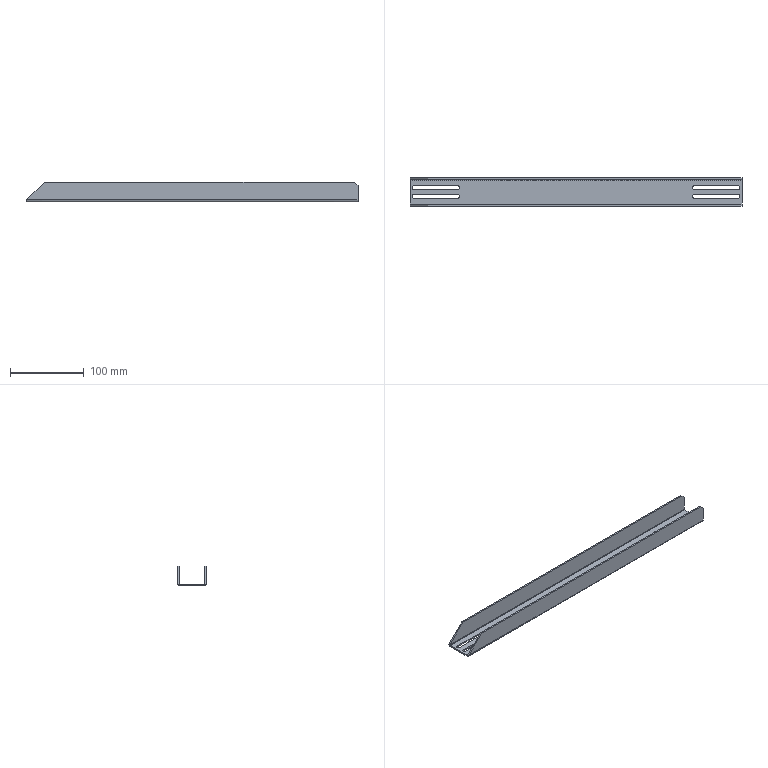Part | NX | 1 solid | 40 faces | box 450 x 38 x 27 mm | volume 74271 mm3 | plane 28 | cylinder 12 | commonest cylinder face diameters 4.5 x8 1.473 x2 5.473 x2
STEP:
#1=CARTESIAN_POINT('',(-160.,-3.75,-2.));
#2=VERTEX_POINT('',#1);
#3=CARTESIAN_POINT('',(-220.,-3.75,-2.));
#4=VERTEX_POINT('',#3);
#5=CARTESIAN_POINT('',(0.,-3.75,-2.));
#6=DIRECTION('',(-1.,0.,0.));
#7=VECTOR('',#6,1000.);
#8=LINE('',#5,#7);
#9=EDGE_CURVE('',#2,#4,#8,.T.);
#10=ORIENTED_EDGE('',*,*,#9,.T.);
#11=CARTESIAN_POINT('',(-220.,-8.25,-2.));
#12=VERTEX_POINT('',#11);
#13=CARTESIAN_POINT('',(-220.,-6.,-2.));
#14=DIRECTION('',(0.,0.,-1.));
#15=DIRECTION('',(-1.,0.,0.));
#16=AXIS2_PLACEMENT_3D('',#13,#14,#15);
#17=CIRCLE('',#16,2.25);
#18=EDGE_CURVE('',#4,#12,#17,.F.);
#19=ORIENTED_EDGE('',*,*,#18,.T.);
#20=CARTESIAN_POINT('',(-160.,-8.25,-2.));
#21=VERTEX_POINT('',#20);
#22=CARTESIAN_POINT('',(0.,-8.25,-2.));
#23=DIRECTION('',(1.,0.,0.));
#24=VECTOR('',#23,1000.);
#25=LINE('',#22,#24);
#26=EDGE_CURVE('',#12,#21,#25,.T.);
#27=ORIENTED_EDGE('',*,*,#26,.T.);
#28=CARTESIAN_POINT('',(-160.,-6.,-2.));
#29=DIRECTION('',(0.,0.,-1.));
#30=DIRECTION('',(-1.,0.,0.));
#31=AXIS2_PLACEMENT_3D('',#28,#29,#30);
#32=CIRCLE('',#31,2.25);
#33=EDGE_CURVE('',#21,#2,#32,.F.);
#34=ORIENTED_EDGE('',*,*,#33,.T.);
#35=EDGE_LOOP('',(#10,#19,#27,#34));
#36=FACE_BOUND('',#35,.T.);
#37=CARTESIAN_POINT('',(-220.,3.75,-2.));
#38=VERTEX_POINT('',#37);
#39=CARTESIAN_POINT('',(-220.,8.25,-2.));
#40=VERTEX_POINT('',#39);
#41=CARTESIAN_POINT('',(-220.,6.,-2.));
#42=DIRECTION('',(0.,0.,-1.));
#43=DIRECTION('',(-1.,0.,0.));
#44=AXIS2_PLACEMENT_3D('',#41,#42,#43);
#45=CIRCLE('',#44,2.25);
#46=EDGE_CURVE('',#38,#40,#45,.T.);
#47=ORIENTED_EDGE('',*,*,#46,.F.);
#48=CARTESIAN_POINT('',(-160.,3.75,-2.));
#49=VERTEX_POINT('',#48);
#50=CARTESIAN_POINT('',(0.,3.75,-2.));
#51=DIRECTION('',(-1.,0.,0.));
#52=VECTOR('',#51,1000.);
#53=LINE('',#50,#52);
#54=EDGE_CURVE('',#49,#38,#53,.T.);
#55=ORIENTED_EDGE('',*,*,#54,.F.);
#56=CARTESIAN_POINT('',(-160.,8.25,-2.));
#57=VERTEX_POINT('',#56);
#58=CARTESIAN_POINT('',(-160.,6.,-2.));
#59=DIRECTION('',(0.,0.,-1.));
#60=DIRECTION('',(-1.,0.,0.));
#61=AXIS2_PLACEMENT_3D('',#58,#59,#60);
#62=CIRCLE('',#61,2.25);
#63=EDGE_CURVE('',#57,#49,#62,.T.);
#64=ORIENTED_EDGE('',*,*,#63,.F.);
#65=CARTESIAN_POINT('',(0.,8.25,-2.));
#66=DIRECTION('',(1.,0.,0.));
#67=VECTOR('',#66,1000.);
#68=LINE('',#65,#67);
#69=EDGE_CURVE('',#40,#57,#68,.T.);
#70=ORIENTED_EDGE('',*,*,#69,.F.);
#71=EDGE_LOOP('',(#47,#55,#64,#70));
#72=FACE_BOUND('',#71,.T.);
#73=CARTESIAN_POINT('',(-225.,16.263,-2.));
#74=VERTEX_POINT('',#73);
#75=CARTESIAN_POINT('',(-225.,-16.263,-2.));
#76=VERTEX_POINT('',#75);
#77=CARTESIAN_POINT('',(-225.,-17.,-2.));
#78=DIRECTION('',(0.,-1.,0.));
#79=VECTOR('',#78,1000.);
#80=LINE('',#77,#79);
#81=EDGE_CURVE('',#74,#76,#80,.T.);
#82=ORIENTED_EDGE('',*,*,#81,.F.);
#83=CARTESIAN_POINT('',(225.,16.263,-2.));
#84=VERTEX_POINT('',#83);
#85=CARTESIAN_POINT('',(-225.,16.263,-2.));
#86=DIRECTION('',(-1.,0.,0.));
#87=VECTOR('',#86,1000.);
#88=LINE('',#85,#87);
#89=EDGE_CURVE('',#74,#84,#88,.F.);
#90=ORIENTED_EDGE('',*,*,#89,.T.);
#91=CARTESIAN_POINT('',(225.,-16.263,-2.));
#92=VERTEX_POINT('',#91);
#93=CARTESIAN_POINT('',(225.,-17.,-2.));
#94=DIRECTION('',(0.,1.,0.));
#95=VECTOR('',#94,1000.);
#96=LINE('',#93,#95);
#97=EDGE_CURVE('',#92,#84,#96,.T.);
#98=ORIENTED_EDGE('',*,*,#97,.F.);
#99=CARTESIAN_POINT('',(225.,-16.263,-2.));
#100=DIRECTION('',(1.,0.,0.));
#101=VECTOR('',#100,1000.);
#102=LINE('',#99,#101);
#103=EDGE_CURVE('',#92,#76,#102,.F.);
#104=ORIENTED_EDGE('',*,*,#103,.T.);
#105=EDGE_LOOP('',(#82,#90,#98,#104));
#106=FACE_BOUND('',#105,.T.);
#107=CARTESIAN_POINT('',(220.,-3.75,-2.));
#108=VERTEX_POINT('',#107);
#109=CARTESIAN_POINT('',(220.,-8.25,-2.));
#110=VERTEX_POINT('',#109);
#111=CARTESIAN_POINT('',(220.,-6.,-2.));
#112=DIRECTION('',(0.,0.,-1.));
#113=DIRECTION('',(-1.,0.,0.));
#114=AXIS2_PLACEMENT_3D('',#111,#112,#113);
#115=CIRCLE('',#114,2.25);
#116=EDGE_CURVE('',#108,#110,#115,.T.);
#117=ORIENTED_EDGE('',*,*,#116,.F.);
#118=CARTESIAN_POINT('',(160.,-3.75,-2.));
#119=VERTEX_POINT('',#118);
#120=CARTESIAN_POINT('',(0.,-3.75,-2.));
#121=DIRECTION('',(1.,0.,0.));
#122=VECTOR('',#121,1000.);
#123=LINE('',#120,#122);
#124=EDGE_CURVE('',#119,#108,#123,.T.);
#125=ORIENTED_EDGE('',*,*,#124,.F.);
#126=CARTESIAN_POINT('',(160.,-8.25,-2.));
#127=VERTEX_POINT('',#126);
#128=CARTESIAN_POINT('',(160.,-6.,-2.));
#129=DIRECTION('',(0.,0.,-1.));
#130=DIRECTION('',(-1.,0.,0.));
#131=AXIS2_PLACEMENT_3D('',#128,#129,#130);
#132=CIRCLE('',#131,2.25);
#133=EDGE_CURVE('',#127,#119,#132,.T.);
#134=ORIENTED_EDGE('',*,*,#133,.F.);
#135=CARTESIAN_POINT('',(0.,-8.25,-2.));
#136=DIRECTION('',(-1.,0.,0.));
#137=VECTOR('',#136,1000.);
#138=LINE('',#135,#137);
#139=EDGE_CURVE('',#110,#127,#138,.T.);
#140=ORIENTED_EDGE('',*,*,#139,.F.);
#141=EDGE_LOOP('',(#117,#125,#134,#140));
#142=FACE_BOUND('',#141,.T.);
#143=CARTESIAN_POINT('',(160.,3.75,-2.));
#144=VERTEX_POINT('',#143);
#145=CARTESIAN_POINT('',(220.,3.75,-2.));
#146=VERTEX_POINT('',#145);
#147=CARTESIAN_POINT('',(0.,3.75,-2.));
#148=DIRECTION('',(1.,0.,0.));
#149=VECTOR('',#148,1000.);
#150=LINE('',#147,#149);
#151=EDGE_CURVE('',#144,#146,#150,.T.);
#152=ORIENTED_EDGE('',*,*,#151,.T.);
#153=CARTESIAN_POINT('',(220.,8.25,-2.));
#154=VERTEX_POINT('',#153);
#155=CARTESIAN_POINT('',(220.,6.,-2.));
#156=DIRECTION('',(0.,0.,-1.));
#157=DIRECTION('',(-1.,0.,0.));
#158=AXIS2_PLACEMENT_3D('',#155,#156,#157);
#159=CIRCLE('',#158,2.25);
#160=EDGE_CURVE('',#146,#154,#159,.F.);
#161=ORIENTED_EDGE('',*,*,#160,.T.);
#162=CARTESIAN_POINT('',(160.,8.25,-2.));
#163=VERTEX_POINT('',#162);
#164=CARTESIAN_POINT('',(0.,8.25,-2.));
#165=DIRECTION('',(-1.,0.,0.));
#166=VECTOR('',#165,1000.);
#167=LINE('',#164,#166);
#168=EDGE_CURVE('',#154,#163,#167,.T.);
#169=ORIENTED_EDGE('',*,*,#168,.T.);
#170=CARTESIAN_POINT('',(160.,6.,-2.));
#171=DIRECTION('',(0.,0.,-1.));
#172=DIRECTION('',(-1.,0.,0.));
#173=AXIS2_PLACEMENT_3D('',#170,#171,#172);
#174=CIRCLE('',#173,2.25);
#175=EDGE_CURVE('',#163,#144,#174,.F.);
#176=ORIENTED_EDGE('',*,*,#175,.T.);
#177=EDGE_LOOP('',(#152,#161,#169,#176));
#178=FACE_BOUND('',#177,.T.);
#179=CARTESIAN_POINT('',(0.,0.,-2.));
#180=DIRECTION('',(0.,0.,-1.));
#181=DIRECTION('',(-1.,0.,0.));
#182=AXIS2_PLACEMENT_3D('',#179,#180,#181);
#183=PLANE('',#182);
#184=ADVANCED_FACE('',(#36,#72,#106,#142,#178),#183,.T.);
#185=CARTESIAN_POINT('',(-220.,-8.25,0.));
#186=VERTEX_POINT('',#185);
#187=CARTESIAN_POINT('',(-220.,-3.75,0.));
#188=VERTEX_POINT('',#187);
#189=CARTESIAN_POINT('',(-220.,-6.,0.));
#190=DIRECTION('',(0.,0.,-1.));
#191=DIRECTION('',(1.,0.,0.));
#192=AXIS2_PLACEMENT_3D('',#189,#190,#191);
#193=CIRCLE('',#192,2.25);
#194=EDGE_CURVE('',#186,#188,#193,.T.);
#195=ORIENTED_EDGE('',*,*,#194,.T.);
#196=CARTESIAN_POINT('',(-160.,-3.75,0.));
#197=VERTEX_POINT('',#196);
#198=CARTESIAN_POINT('',(-220.,-3.75,0.));
#199=DIRECTION('',(1.,0.,0.));
#200=VECTOR('',#199,1000.);
#201=LINE('',#198,#200);
#202=EDGE_CURVE('',#188,#197,#201,.T.);
#203=ORIENTED_EDGE('',*,*,#202,.T.);
#204=CARTESIAN_POINT('',(-160.,-8.25,0.));
#205=VERTEX_POINT('',#204);
#206=CARTESIAN_POINT('',(-160.,-6.,0.));
#207=DIRECTION('',(0.,0.,-1.));
#208=DIRECTION('',(1.,0.,0.));
#209=AXIS2_PLACEMENT_3D('',#206,#207,#208);
#210=CIRCLE('',#209,2.25);
#211=EDGE_CURVE('',#197,#205,#210,.T.);
#212=ORIENTED_EDGE('',*,*,#211,.T.);
#213=CARTESIAN_POINT('',(-220.,-8.25,0.));
#214=DIRECTION('',(-1.,0.,0.));
#215=VECTOR('',#214,1000.);
#216=LINE('',#213,#215);
#217=EDGE_CURVE('',#205,#186,#216,.T.);
#218=ORIENTED_EDGE('',*,*,#217,.T.);
#219=EDGE_LOOP('',(#195,#203,#212,#218));
#220=FACE_BOUND('',#219,.T.);
#221=CARTESIAN_POINT('',(-220.,3.75,0.));
#222=VERTEX_POINT('',#221);
#223=CARTESIAN_POINT('',(-160.,3.75,0.));
#224=VERTEX_POINT('',#223);
#225=CARTESIAN_POINT('',(-220.,3.75,0.));
#226=DIRECTION('',(1.,0.,0.));
#227=VECTOR('',#226,1000.);
#228=LINE('',#225,#227);
#229=EDGE_CURVE('',#222,#224,#228,.T.);
#230=ORIENTED_EDGE('',*,*,#229,.F.);
#231=CARTESIAN_POINT('',(-220.,8.25,0.));
#232=VERTEX_POINT('',#231);
#233=CARTESIAN_POINT('',(-220.,6.,0.));
#234=DIRECTION('',(0.,0.,1.));
#235=DIRECTION('',(1.,0.,0.));
#236=AXIS2_PLACEMENT_3D('',#233,#234,#235);
#237=CIRCLE('',#236,2.25);
#238=EDGE_CURVE('',#232,#222,#237,.T.);
#239=ORIENTED_EDGE('',*,*,#238,.F.);
#240=CARTESIAN_POINT('',(-160.,8.25,0.));
#241=VERTEX_POINT('',#240);
#242=CARTESIAN_POINT('',(-220.,8.25,0.));
#243=DIRECTION('',(-1.,0.,0.));
#244=VECTOR('',#243,1000.);
#245=LINE('',#242,#244);
#246=EDGE_CURVE('',#241,#232,#245,.T.);
#247=ORIENTED_EDGE('',*,*,#246,.F.);
#248=CARTESIAN_POINT('',(-160.,6.,0.));
#249=DIRECTION('',(0.,0.,1.));
#250=DIRECTION('',(1.,0.,0.));
#251=AXIS2_PLACEMENT_3D('',#248,#249,#250);
#252=CIRCLE('',#251,2.25);
#253=EDGE_CURVE('',#224,#241,#252,.T.);
#254=ORIENTED_EDGE('',*,*,#253,.F.);
#255=EDGE_LOOP('',(#230,#239,#247,#254));
#256=FACE_BOUND('',#255,.T.);
#257=CARTESIAN_POINT('',(-225.,16.263,0.));
#258=VERTEX_POINT('',#257);
#259=CARTESIAN_POINT('',(225.,16.263,0.));
#260=VERTEX_POINT('',#259);
#261=CARTESIAN_POINT('',(-225.,16.263,0.));
#262=DIRECTION('',(-1.,0.,0.));
#263=VECTOR('',#262,1000.);
#264=LINE('',#261,#263);
#265=EDGE_CURVE('',#258,#260,#264,.F.);
#266=ORIENTED_EDGE('',*,*,#265,.F.);
#267=CARTESIAN_POINT('',(-225.,-16.263,0.));
#268=VERTEX_POINT('',#267);
#269=CARTESIAN_POINT('',(-225.,-17.,0.));
#270=DIRECTION('',(0.,-1.,0.));
#271=VECTOR('',#270,1000.);
#272=LINE('',#269,#271);
#273=EDGE_CURVE('',#258,#268,#272,.T.);
#274=ORIENTED_EDGE('',*,*,#273,.T.);
#275=CARTESIAN_POINT('',(225.,-16.263,0.));
#276=VERTEX_POINT('',#275);
#277=CARTESIAN_POINT('',(225.,-16.263,0.));
#278=DIRECTION('',(1.,0.,0.));
#279=VECTOR('',#278,1000.);
#280=LINE('',#277,#279);
#281=EDGE_CURVE('',#276,#268,#280,.F.);
#282=ORIENTED_EDGE('',*,*,#281,.F.);
#283=CARTESIAN_POINT('',(225.,-17.,0.));
#284=DIRECTION('',(0.,1.,0.));
#285=VECTOR('',#284,1000.);
#286=LINE('',#283,#285);
#287=EDGE_CURVE('',#276,#260,#286,.T.);
#288=ORIENTED_EDGE('',*,*,#287,.T.);
#289=EDGE_LOOP('',(#266,#274,#282,#288));
#290=FACE_BOUND('',#289,.T.);
#291=CARTESIAN_POINT('',(220.,-3.75,0.));
#292=VERTEX_POINT('',#291);
#293=CARTESIAN_POINT('',(160.,-3.75,0.));
#294=VERTEX_POINT('',#293);
#295=CARTESIAN_POINT('',(220.,-3.75,0.));
#296=DIRECTION('',(-1.,0.,0.));
#297=VECTOR('',#296,1000.);
#298=LINE('',#295,#297);
#299=EDGE_CURVE('',#292,#294,#298,.T.);
#300=ORIENTED_EDGE('',*,*,#299,.F.);
#301=CARTESIAN_POINT('',(220.,-8.25,0.));
#302=VERTEX_POINT('',#301);
#303=CARTESIAN_POINT('',(220.,-6.,0.));
#304=DIRECTION('',(0.,0.,1.));
#305=DIRECTION('',(-1.,0.,0.));
#306=AXIS2_PLACEMENT_3D('',#303,#304,#305);
#307=CIRCLE('',#306,2.25);
#308=EDGE_CURVE('',#302,#292,#307,.T.);
#309=ORIENTED_EDGE('',*,*,#308,.F.);
#310=CARTESIAN_POINT('',(160.,-8.25,0.));
#311=VERTEX_POINT('',#310);
#312=CARTESIAN_POINT('',(220.,-8.25,0.));
#313=DIRECTION('',(1.,0.,0.));
#314=VECTOR('',#313,1000.);
#315=LINE('',#312,#314);
#316=EDGE_CURVE('',#311,#302,#315,.T.);
#317=ORIENTED_EDGE('',*,*,#316,.F.);
#318=CARTESIAN_POINT('',(160.,-6.,0.));
#319=DIRECTION('',(0.,0.,1.));
#320=DIRECTION('',(-1.,0.,0.));
#321=AXIS2_PLACEMENT_3D('',#318,#319,#320);
#322=CIRCLE('',#321,2.25);
#323=EDGE_CURVE('',#294,#311,#322,.T.);
#324=ORIENTED_EDGE('',*,*,#323,.F.);
#325=EDGE_LOOP('',(#300,#309,#317,#324));
#326=FACE_BOUND('',#325,.T.);
#327=CARTESIAN_POINT('',(220.,8.25,0.));
#328=VERTEX_POINT('',#327);
#329=CARTESIAN_POINT('',(220.,3.75,0.));
#330=VERTEX_POINT('',#329);
#331=CARTESIAN_POINT('',(220.,6.,0.));
#332=DIRECTION('',(0.,0.,-1.));
#333=DIRECTION('',(-1.,0.,0.));
#334=AXIS2_PLACEMENT_3D('',#331,#332,#333);
#335=CIRCLE('',#334,2.25);
#336=EDGE_CURVE('',#328,#330,#335,.T.);
#337=ORIENTED_EDGE('',*,*,#336,.T.);
#338=CARTESIAN_POINT('',(160.,3.75,0.));
#339=VERTEX_POINT('',#338);
#340=CARTESIAN_POINT('',(220.,3.75,0.));
#341=DIRECTION('',(-1.,0.,0.));
#342=VECTOR('',#341,1000.);
#343=LINE('',#340,#342);
#344=EDGE_CURVE('',#330,#339,#343,.T.);
#345=ORIENTED_EDGE('',*,*,#344,.T.);
#346=CARTESIAN_POINT('',(160.,8.25,0.));
#347=VERTEX_POINT('',#346);
#348=CARTESIAN_POINT('',(160.,6.,0.));
#349=DIRECTION('',(0.,0.,-1.));
#350=DIRECTION('',(-1.,0.,0.));
#351=AXIS2_PLACEMENT_3D('',#348,#349,#350);
#352=CIRCLE('',#351,2.25);
#353=EDGE_CURVE('',#339,#347,#352,.T.);
#354=ORIENTED_EDGE('',*,*,#353,.T.);
#355=CARTESIAN_POINT('',(220.,8.25,0.));
#356=DIRECTION('',(1.,0.,0.));
#357=VECTOR('',#356,1000.);
#358=LINE('',#355,#357);
#359=EDGE_CURVE('',#347,#328,#358,.T.);
#360=ORIENTED_EDGE('',*,*,#359,.T.);
#361=EDGE_LOOP('',(#337,#345,#354,#360));
#362=FACE_BOUND('',#361,.T.);
#363=CARTESIAN_POINT('',(0.,0.,0.));
#364=DIRECTION('',(0.,0.,-1.));
#365=DIRECTION('',(-1.,0.,0.));
#366=AXIS2_PLACEMENT_3D('',#363,#364,#365);
#367=PLANE('',#366);
#368=ADVANCED_FACE('',(#220,#256,#290,#326,#362),#367,.F.);
#369=ORIENTED_EDGE('',*,*,#273,.F.);
#370=CARTESIAN_POINT('',(-225.,16.263,0.));
#371=DIRECTION('',(0.,0.,-1.));
#372=VECTOR('',#371,1000.);
#373=LINE('',#370,#372);
#374=EDGE_CURVE('',#258,#74,#373,.T.);
#375=ORIENTED_EDGE('',*,*,#374,.T.);
#376=ORIENTED_EDGE('',*,*,#81,.T.);
#377=CARTESIAN_POINT('',(-225.,-16.263,0.));
#378=DIRECTION('',(0.,0.,-1.));
#379=VECTOR('',#378,1000.);
#380=LINE('',#377,#379);
#381=EDGE_CURVE('',#268,#76,#380,.T.);
#382=ORIENTED_EDGE('',*,*,#381,.F.);
#383=EDGE_LOOP('',(#369,#375,#376,#382));
#384=FACE_BOUND('',#383,.T.);
#385=CARTESIAN_POINT('',(-225.,-17.,-2.));
#386=DIRECTION('',(-1.,0.,0.));
#387=DIRECTION('',(0.,0.,1.));
#388=AXIS2_PLACEMENT_3D('',#385,#386,#387);
#389=PLANE('',#388);
#390=ADVANCED_FACE('',(#384),#389,.T.);
#391=CARTESIAN_POINT('',(225.,16.263,0.));
#392=DIRECTION('',(0.,0.,-1.));
#393=VECTOR('',#392,1000.);
#394=LINE('',#391,#393);
#395=EDGE_CURVE('',#260,#84,#394,.T.);
#396=ORIENTED_EDGE('',*,*,#395,.F.);
#397=ORIENTED_EDGE('',*,*,#287,.F.);
#398=CARTESIAN_POINT('',(225.,-16.263,0.));
#399=DIRECTION('',(0.,0.,-1.));
#400=VECTOR('',#399,1000.);
#401=LINE('',#398,#400);
#402=EDGE_CURVE('',#276,#92,#401,.T.);
#403=ORIENTED_EDGE('',*,*,#402,.T.);
#404=ORIENTED_EDGE('',*,*,#97,.T.);
#405=EDGE_LOOP('',(#396,#397,#403,#404));
#406=FACE_BOUND('',#405,.T.);
#407=CARTESIAN_POINT('',(225.,-17.,-2.));
#408=DIRECTION('',(1.,0.,0.));
#409=DIRECTION('',(0.,0.,-1.));
#410=AXIS2_PLACEMENT_3D('',#407,#408,#409);
#411=PLANE('',#410);
#412=ADVANCED_FACE('',(#406),#411,.T.);
#413=CARTESIAN_POINT('',(-225.,-18.899,0.));
#414=VERTEX_POINT('',#413);
#415=CARTESIAN_POINT('',(-225.,-16.263,0.7366));
#416=DIRECTION('',(1.,0.,0.));
#417=DIRECTION('',(0.,0.,-1.));
#418=AXIS2_PLACEMENT_3D('',#415,#416,#417);
#419=CIRCLE('',#418,2.737);
#420=EDGE_CURVE('',#76,#414,#419,.F.);
#421=ORIENTED_EDGE('',*,*,#420,.T.);
#422=CARTESIAN_POINT('',(-225.,-17.,0.));
#423=DIRECTION('',(0.,1.,0.));
#424=VECTOR('',#423,1000.);
#425=LINE('',#422,#424);
#426=EDGE_CURVE('',#414,#268,#425,.T.);
#427=ORIENTED_EDGE('',*,*,#426,.T.);
#428=ORIENTED_EDGE('',*,*,#381,.T.);
#429=EDGE_LOOP('',(#421,#427,#428));
#430=FACE_BOUND('',#429,.T.);
#431=CARTESIAN_POINT('',(-225.,-16.263,0.7366));
#432=DIRECTION('',(-1.,0.,0.));
#433=DIRECTION('',(0.,0.,1.));
#434=AXIS2_PLACEMENT_3D('',#431,#432,#433);
#435=PLANE('',#434);
#436=ADVANCED_FACE('',(#430),#435,.T.);
#437=CARTESIAN_POINT('',(225.,-17.,0.7366));
#438=VERTEX_POINT('',#437);
#439=CARTESIAN_POINT('',(225.,-16.263,0.7366));
#440=DIRECTION('',(1.,0.,0.));
#441=DIRECTION('',(0.,0.,-1.));
#442=AXIS2_PLACEMENT_3D('',#439,#440,#441);
#443=CIRCLE('',#442,0.7366);
#444=EDGE_CURVE('',#438,#276,#443,.T.);
#445=ORIENTED_EDGE('',*,*,#444,.F.);
#446=CARTESIAN_POINT('',(225.,-19.,0.7366));
#447=VERTEX_POINT('',#446);
#448=CARTESIAN_POINT('',(225.,-17.,0.7366));
#449=DIRECTION('',(0.,-1.,0.));
#450=VECTOR('',#449,1000.);
#451=LINE('',#448,#450);
#452=EDGE_CURVE('',#438,#447,#451,.T.);
#453=ORIENTED_EDGE('',*,*,#452,.T.);
#454=CARTESIAN_POINT('',(225.,-16.263,0.7366));
#455=DIRECTION('',(1.,0.,0.));
#456=DIRECTION('',(0.,0.,-1.));
#457=AXIS2_PLACEMENT_3D('',#454,#455,#456);
#458=CIRCLE('',#457,2.737);
#459=EDGE_CURVE('',#447,#92,#458,.T.);
#460=ORIENTED_EDGE('',*,*,#459,.T.);
#461=ORIENTED_EDGE('',*,*,#402,.F.);
#462=EDGE_LOOP('',(#445,#453,#460,#461));
#463=FACE_BOUND('',#462,.T.);
#464=CARTESIAN_POINT('',(225.,-16.263,0.7366));
#465=DIRECTION('',(-1.,0.,0.));
#466=DIRECTION('',(0.,0.,1.));
#467=AXIS2_PLACEMENT_3D('',#464,#465,#466);
#468=PLANE('',#467);
#469=ADVANCED_FACE('',(#463),#468,.F.);
#470=CARTESIAN_POINT('',(-224.263,-19.,0.7366));
#471=VERTEX_POINT('',#470);
#472=CARTESIAN_POINT('',(0.,-19.,0.7366));
#473=DIRECTION('',(-1.,0.,0.));
#474=VECTOR('',#473,1000.);
#475=LINE('',#472,#474);
#476=EDGE_CURVE('',#447,#471,#475,.T.);
#477=ORIENTED_EDGE('',*,*,#476,.T.);
#478=CARTESIAN_POINT('',(-224.263,-16.263,0.7366));
#479=DIRECTION('',(-0.7071,0.,0.7071));
#480=DIRECTION('',(0.7071,0.,0.7071));
#481=AXIS2_PLACEMENT_3D('',#478,#479,#480);
#482=ELLIPSE('',#481,3.87,2.737);
#483=EDGE_CURVE('',#471,#414,#482,.F.);
#484=ORIENTED_EDGE('',*,*,#483,.T.);
#485=ORIENTED_EDGE('',*,*,#420,.F.);
#486=ORIENTED_EDGE('',*,*,#103,.F.);
#487=ORIENTED_EDGE('',*,*,#459,.F.);
#488=EDGE_LOOP('',(#477,#484,#485,#486,#487));
#489=FACE_BOUND('',#488,.T.);
#490=CARTESIAN_POINT('',(225.,-16.263,0.7366));
#491=DIRECTION('',(1.,0.,0.));
#492=DIRECTION('',(0.,-1.,0.));
#493=AXIS2_PLACEMENT_3D('',#490,#491,#492);
#494=CYLINDRICAL_SURFACE('',#493,2.737);
#495=ADVANCED_FACE('',(#489),#494,.T.);
#496=ORIENTED_EDGE('',*,*,#281,.T.);
#497=CARTESIAN_POINT('',(-224.263,-17.,0.7366));
#498=VERTEX_POINT('',#497);
#499=CARTESIAN_POINT('',(-224.263,-16.263,0.7366));
#500=DIRECTION('',(-0.7071,0.,0.7071));
#501=DIRECTION('',(0.7071,0.,0.7071));
#502=AXIS2_PLACEMENT_3D('',#499,#500,#501);
#503=ELLIPSE('',#502,1.042,0.7366);
#504=EDGE_CURVE('',#268,#498,#503,.T.);
#505=ORIENTED_EDGE('',*,*,#504,.T.);
#506=CARTESIAN_POINT('',(-225.,-17.,0.7366));
#507=DIRECTION('',(1.,0.,0.));
#508=VECTOR('',#507,1000.);
#509=LINE('',#506,#508);
#510=EDGE_CURVE('',#498,#438,#509,.T.);
#511=ORIENTED_EDGE('',*,*,#510,.T.);
#512=ORIENTED_EDGE('',*,*,#444,.T.);
#513=EDGE_LOOP('',(#496,#505,#511,#512));
#514=FACE_BOUND('',#513,.T.);
#515=CARTESIAN_POINT('',(225.,-16.263,0.7366));
#516=DIRECTION('',(1.,0.,0.));
#517=DIRECTION('',(0.,-1.,0.));
#518=AXIS2_PLACEMENT_3D('',#515,#516,#517);
#519=CYLINDRICAL_SURFACE('',#518,0.7366);
#520=ADVANCED_FACE('',(#514),#519,.F.);
#521=CARTESIAN_POINT('',(225.,-17.,20.));
#522=VERTEX_POINT('',#521);
#523=CARTESIAN_POINT('',(225.,-17.,25.));
#524=DIRECTION('',(0.,0.,1.));
#525=VECTOR('',#524,1000.);
#526=LINE('',#523,#525);
#527=EDGE_CURVE('',#438,#522,#526,.T.);
#528=ORIENTED_EDGE('',*,*,#527,.T.);
#529=CARTESIAN_POINT('',(225.,-19.,20.));
#530=VERTEX_POINT('',#529);
#531=CARTESIAN_POINT('',(225.,-19.,20.));
#532=DIRECTION('',(0.,-1.,0.));
#533=VECTOR('',#532,1000.);
#534=LINE('',#531,#533);
#535=EDGE_CURVE('',#522,#530,#534,.T.);
#536=ORIENTED_EDGE('',*,*,#535,.T.);
#537=CARTESIAN_POINT('',(225.,-19.,25.));
#538=DIRECTION('',(0.,0.,1.));
#539=VECTOR('',#538,1000.);
#540=LINE('',#537,#539);
#541=EDGE_CURVE('',#447,#530,#540,.T.);
#542=ORIENTED_EDGE('',*,*,#541,.F.);
#543=ORIENTED_EDGE('',*,*,#452,.F.);
#544=EDGE_LOOP('',(#528,#536,#542,#543));
#545=FACE_BOUND('',#544,.T.);
#546=CARTESIAN_POINT('',(225.,-19.,25.));
#547=DIRECTION('',(-1.,0.,0.));
#548=DIRECTION('',(0.,0.,1.));
#549=AXIS2_PLACEMENT_3D('',#546,#547,#548);
#550=PLANE('',#549);
#551=ADVANCED_FACE('',(#545),#550,.F.);
#552=ORIENTED_EDGE('',*,*,#541,.T.);
#553=CARTESIAN_POINT('',(220.,-19.,25.));
#554=VERTEX_POINT('',#553);
#555=CARTESIAN_POINT('',(220.,-19.,25.));
#556=DIRECTION('',(0.7071,0.,-0.7071));
#557=VECTOR('',#556,1000.);
#558=LINE('',#555,#557);
#559=EDGE_CURVE('',#530,#554,#558,.F.);
#560=ORIENTED_EDGE('',*,*,#559,.T.);
#561=CARTESIAN_POINT('',(-200.,-19.,25.));
#562=VERTEX_POINT('',#561);
#563=CARTESIAN_POINT('',(-225.,-19.,25.));
#564=DIRECTION('',(-1.,0.,0.));
#565=VECTOR('',#564,1000.);
#566=LINE('',#563,#565);
#567=EDGE_CURVE('',#554,#562,#566,.T.);
#568=ORIENTED_EDGE('',*,*,#567,.T.);
#569=CARTESIAN_POINT('',(-225.,-19.,0.));
#570=DIRECTION('',(-0.7071,0.,-0.7071));
#571=VECTOR('',#570,1000.);
#572=LINE('',#569,#571);
#573=EDGE_CURVE('',#562,#471,#572,.T.);
#574=ORIENTED_EDGE('',*,*,#573,.T.);
#575=ORIENTED_EDGE('',*,*,#476,.F.);
#576=EDGE_LOOP('',(#552,#560,#568,#574,#575));
#577=FACE_BOUND('',#576,.T.);
#578=CARTESIAN_POINT('',(0.,-19.,0.));
#579=DIRECTION('',(0.,1.,0.));
#580=DIRECTION('',(0.,0.,1.));
#581=AXIS2_PLACEMENT_3D('',#578,#579,#580);
#582=PLANE('',#581);
#583=ADVANCED_FACE('',(#577),#582,.F.);
#584=CARTESIAN_POINT('',(220.,-17.,25.));
#585=VERTEX_POINT('',#584);
#586=CARTESIAN_POINT('',(-200.,-17.,25.));
#587=VERTEX_POINT('',#586);
#588=CARTESIAN_POINT('',(-225.,-17.,25.));
#589=DIRECTION('',(-1.,0.,0.));
#590=VECTOR('',#589,1000.);
#591=LINE('',#588,#590);
#592=EDGE_CURVE('',#585,#587,#591,.T.);
#593=ORIENTED_EDGE('',*,*,#592,.F.);
#594=CARTESIAN_POINT('',(122.5,-17.,122.5));
#595=DIRECTION('',(-0.7071,0.,0.7071));
#596=VECTOR('',#595,1000.);
#597=LINE('',#594,#596);
#598=EDGE_CURVE('',#585,#522,#597,.F.);
#599=ORIENTED_EDGE('',*,*,#598,.T.);
#600=ORIENTED_EDGE('',*,*,#527,.F.);
#601=ORIENTED_EDGE('',*,*,#510,.F.);
#602=CARTESIAN_POINT('',(-112.5,-17.,112.5));
#603=DIRECTION('',(0.7071,0.,0.7071));
#604=VECTOR('',#603,1000.);
#605=LINE('',#602,#604);
#606=EDGE_CURVE('',#498,#587,#605,.T.);
#607=ORIENTED_EDGE('',*,*,#606,.T.);
#608=EDGE_LOOP('',(#593,#599,#600,#601,#607));
#609=FACE_BOUND('',#608,.T.);
#610=CARTESIAN_POINT('',(0.,-17.,0.));
#611=DIRECTION('',(0.,1.,0.));
#612=DIRECTION('',(0.,0.,1.));
#613=AXIS2_PLACEMENT_3D('',#610,#611,#612);
#614=PLANE('',#613);
#615=ADVANCED_FACE('',(#609),#614,.T.);
#616=ORIENTED_EDGE('',*,*,#567,.F.);
#617=CARTESIAN_POINT('',(220.,-19.,25.));
#618=DIRECTION('',(0.,1.,0.));
#619=VECTOR('',#618,1000.);
#620=LINE('',#617,#619);
#621=EDGE_CURVE('',#554,#585,#620,.T.);
#622=ORIENTED_EDGE('',*,*,#621,.T.);
#623=ORIENTED_EDGE('',*,*,#592,.T.);
#624=CARTESIAN_POINT('',(-200.,-19.,25.));
#625=DIRECTION('',(0.,-1.,0.));
#626=VECTOR('',#625,1000.);
#627=LINE('',#624,#626);
#628=EDGE_CURVE('',#587,#562,#627,.T.);
#629=ORIENTED_EDGE('',*,*,#628,.T.);
#630=EDGE_LOOP('',(#616,#622,#623,#629));
#631=FACE_BOUND('',#630,.T.);
#632=CARTESIAN_POINT('',(-225.,-19.,25.));
#633=DIRECTION('',(0.,0.,-1.));
#634=DIRECTION('',(0.,1.,0.));
#635=AXIS2_PLACEMENT_3D('',#632,#633,#634);
#636=PLANE('',#635);
#637=ADVANCED_FACE('',(#631),#636,.F.);
#638=CARTESIAN_POINT('',(225.,17.,0.7366));
#639=VERTEX_POINT('',#638);
#640=CARTESIAN_POINT('',(225.,19.,0.7366));
#641=VERTEX_POINT('',#640);
#642=CARTESIAN_POINT('',(225.,17.,0.7366));
#643=DIRECTION('',(0.,1.,0.));
#644=VECTOR('',#643,1000.);
#645=LINE('',#642,#644);
#646=EDGE_CURVE('',#639,#641,#645,.T.);
#647=ORIENTED_EDGE('',*,*,#646,.F.);
#648=CARTESIAN_POINT('',(225.,16.263,0.7366));
#649=DIRECTION('',(-1.,0.,0.));
#650=DIRECTION('',(0.,0.,1.));
#651=AXIS2_PLACEMENT_3D('',#648,#649,#650);
#652=CIRCLE('',#651,0.7366);
#653=EDGE_CURVE('',#260,#639,#652,.F.);
#654=ORIENTED_EDGE('',*,*,#653,.F.);
#655=ORIENTED_EDGE('',*,*,#395,.T.);
#656=CARTESIAN_POINT('',(225.,16.263,0.7366));
#657=DIRECTION('',(-1.,0.,0.));
#658=DIRECTION('',(0.,0.,1.));
#659=AXIS2_PLACEMENT_3D('',#656,#657,#658);
#660=CIRCLE('',#659,2.737);
#661=EDGE_CURVE('',#84,#641,#660,.F.);
#662=ORIENTED_EDGE('',*,*,#661,.T.);
#663=EDGE_LOOP('',(#647,#654,#655,#662));
#664=FACE_BOUND('',#663,.T.);
#665=CARTESIAN_POINT('',(225.,16.263,0.7366));
#666=DIRECTION('',(1.,0.,0.));
#667=DIRECTION('',(0.,0.,-1.));
#668=AXIS2_PLACEMENT_3D('',#665,#666,#667);
#669=PLANE('',#668);
#670=ADVANCED_FACE('',(#664),#669,.T.);
#671=ORIENTED_EDGE('',*,*,#374,.F.);
#672=CARTESIAN_POINT('',(-225.,18.899,0.));
#673=VERTEX_POINT('',#672);
#674=CARTESIAN_POINT('',(-225.,19.,0.));
#675=DIRECTION('',(0.,-1.,0.));
#676=VECTOR('',#675,1000.);
#677=LINE('',#674,#676);
#678=EDGE_CURVE('',#258,#673,#677,.F.);
#679=ORIENTED_EDGE('',*,*,#678,.T.);
#680=CARTESIAN_POINT('',(-225.,16.263,0.7366));
#681=DIRECTION('',(-1.,0.,0.));
#682=DIRECTION('',(0.,0.,1.));
#683=AXIS2_PLACEMENT_3D('',#680,#681,#682);
#684=CIRCLE('',#683,2.737);
#685=EDGE_CURVE('',#673,#74,#684,.T.);
#686=ORIENTED_EDGE('',*,*,#685,.T.);
#687=EDGE_LOOP('',(#671,#679,#686));
#688=FACE_BOUND('',#687,.T.);
#689=CARTESIAN_POINT('',(-225.,16.263,0.7366));
#690=DIRECTION('',(1.,0.,0.));
#691=DIRECTION('',(0.,0.,-1.));
#692=AXIS2_PLACEMENT_3D('',#689,#690,#691);
#693=PLANE('',#692);
#694=ADVANCED_FACE('',(#688),#693,.F.);
#695=ORIENTED_EDGE('',*,*,#685,.F.);
#696=CARTESIAN_POINT('',(-224.263,19.,0.7366));
#697=VERTEX_POINT('',#696);
#698=CARTESIAN_POINT('',(-224.263,16.263,0.7366));
#699=DIRECTION('',(0.7071,0.,-0.7071));
#700=DIRECTION('',(-0.7071,0.,-0.7071));
#701=AXIS2_PLACEMENT_3D('',#698,#699,#700);
#702=ELLIPSE('',#701,3.87,2.737);
#703=EDGE_CURVE('',#673,#697,#702,.T.);
#704=ORIENTED_EDGE('',*,*,#703,.T.);
#705=CARTESIAN_POINT('',(0.,19.,0.7366));
#706=DIRECTION('',(1.,0.,0.));
#707=VECTOR('',#706,1000.);
#708=LINE('',#705,#707);
#709=EDGE_CURVE('',#697,#641,#708,.T.);
#710=ORIENTED_EDGE('',*,*,#709,.T.);
#711=ORIENTED_EDGE('',*,*,#661,.F.);
#712=ORIENTED_EDGE('',*,*,#89,.F.);
#713=EDGE_LOOP('',(#695,#704,#710,#711,#712));
#714=FACE_BOUND('',#713,.T.);
#715=CARTESIAN_POINT('',(-225.,16.263,0.7366));
#716=DIRECTION('',(-1.,0.,0.));
#717=DIRECTION('',(0.,1.,0.));
#718=AXIS2_PLACEMENT_3D('',#715,#716,#717);
#719=CYLINDRICAL_SURFACE('',#718,2.737);
#720=ADVANCED_FACE('',(#714),#719,.T.);
#721=CARTESIAN_POINT('',(-224.263,17.,0.7366));
#722=VERTEX_POINT('',#721);
#723=CARTESIAN_POINT('',(225.,17.,0.7366));
#724=DIRECTION('',(-1.,0.,0.));
#725=VECTOR('',#724,1000.);
#726=LINE('',#723,#725);
#727=EDGE_CURVE('',#639,#722,#726,.T.);
#728=ORIENTED_EDGE('',*,*,#727,.T.);
#729=CARTESIAN_POINT('',(-224.263,16.263,0.7366));
#730=DIRECTION('',(0.7071,0.,-0.7071));
#731=DIRECTION('',(-0.7071,0.,-0.7071));
#732=AXIS2_PLACEMENT_3D('',#729,#730,#731);
#733=ELLIPSE('',#732,1.042,0.7366);
#734=EDGE_CURVE('',#722,#258,#733,.F.);
#735=ORIENTED_EDGE('',*,*,#734,.T.);
#736=ORIENTED_EDGE('',*,*,#265,.T.);
#737=ORIENTED_EDGE('',*,*,#653,.T.);
#738=EDGE_LOOP('',(#728,#735,#736,#737));
#739=FACE_BOUND('',#738,.T.);
#740=CARTESIAN_POINT('',(-225.,16.263,0.7366));
#741=DIRECTION('',(-1.,0.,0.));
#742=DIRECTION('',(0.,1.,0.));
#743=AXIS2_PLACEMENT_3D('',#740,#741,#742);
#744=CYLINDRICAL_SURFACE('',#743,0.7366);
#745=ADVANCED_FACE('',(#739),#744,.F.);
#746=CARTESIAN_POINT('',(225.,19.,20.));
#747=VERTEX_POINT('',#746);
#748=CARTESIAN_POINT('',(225.,19.,0.));
#749=DIRECTION('',(0.,0.,-1.));
#750=VECTOR('',#749,1000.);
#751=LINE('',#748,#750);
#752=EDGE_CURVE('',#747,#641,#751,.T.);
#753=ORIENTED_EDGE('',*,*,#752,.F.);
#754=CARTESIAN_POINT('',(225.,17.,20.));
#755=VERTEX_POINT('',#754);
#756=CARTESIAN_POINT('',(225.,19.,20.));
#757=DIRECTION('',(0.,-1.,0.));
#758=VECTOR('',#757,1000.);
#759=LINE('',#756,#758);
#760=EDGE_CURVE('',#747,#755,#759,.T.);
#761=ORIENTED_EDGE('',*,*,#760,.T.);
#762=CARTESIAN_POINT('',(225.,17.,0.));
#763=DIRECTION('',(0.,0.,-1.));
#764=VECTOR('',#763,1000.);
#765=LINE('',#762,#764);
#766=EDGE_CURVE('',#755,#639,#765,.T.);
#767=ORIENTED_EDGE('',*,*,#766,.T.);
#768=ORIENTED_EDGE('',*,*,#646,.T.);
#769=EDGE_LOOP('',(#753,#761,#767,#768));
#770=FACE_BOUND('',#769,.T.);
#771=CARTESIAN_POINT('',(225.,19.,0.));
#772=DIRECTION('',(-1.,0.,0.));
#773=DIRECTION('',(0.,0.,1.));
#774=AXIS2_PLACEMENT_3D('',#771,#772,#773);
#775=PLANE('',#774);
#776=ADVANCED_FACE('',(#770),#775,.F.);
#777=CARTESIAN_POINT('',(-200.,19.,25.));
#778=VERTEX_POINT('',#777);
#779=CARTESIAN_POINT('',(220.,19.,25.));
#780=VERTEX_POINT('',#779);
#781=CARTESIAN_POINT('',(225.,19.,25.));
#782=DIRECTION('',(1.,0.,0.));
#783=VECTOR('',#782,1000.);
#784=LINE('',#781,#783);
#785=EDGE_CURVE('',#778,#780,#784,.T.);
#786=ORIENTED_EDGE('',*,*,#785,.T.);
#787=CARTESIAN_POINT('',(225.,19.,20.));
#788=DIRECTION('',(-0.7071,0.,0.7071));
#789=VECTOR('',#788,1000.);
#790=LINE('',#787,#789);
#791=EDGE_CURVE('',#780,#747,#790,.F.);
#792=ORIENTED_EDGE('',*,*,#791,.T.);
#793=ORIENTED_EDGE('',*,*,#752,.T.);
#794=ORIENTED_EDGE('',*,*,#709,.F.);
#795=CARTESIAN_POINT('',(-200.,19.,25.));
#796=DIRECTION('',(-0.7071,0.,-0.7071));
#797=VECTOR('',#796,1000.);
#798=LINE('',#795,#797);
#799=EDGE_CURVE('',#697,#778,#798,.F.);
#800=ORIENTED_EDGE('',*,*,#799,.T.);
#801=EDGE_LOOP('',(#786,#792,#793,#794,#800));
#802=FACE_BOUND('',#801,.T.);
#803=CARTESIAN_POINT('',(0.,19.,0.));
#804=DIRECTION('',(0.,-1.,0.));
#805=DIRECTION('',(0.,0.,-1.));
#806=AXIS2_PLACEMENT_3D('',#803,#804,#805);
#807=PLANE('',#806);
#808=ADVANCED_FACE('',(#802),#807,.F.);
#809=ORIENTED_EDGE('',*,*,#766,.F.);
#810=CARTESIAN_POINT('',(220.,17.,25.));
#811=VERTEX_POINT('',#810);
#812=CARTESIAN_POINT('',(122.5,17.,122.5));
#813=DIRECTION('',(0.7071,0.,-0.7071));
#814=VECTOR('',#813,1000.);
#815=LINE('',#812,#814);
#816=EDGE_CURVE('',#755,#811,#815,.F.);
#817=ORIENTED_EDGE('',*,*,#816,.T.);
#818=CARTESIAN_POINT('',(-200.,17.,25.));
#819=VERTEX_POINT('',#818);
#820=CARTESIAN_POINT('',(225.,17.,25.));
#821=DIRECTION('',(1.,0.,0.));
#822=VECTOR('',#821,1000.);
#823=LINE('',#820,#822);
#824=EDGE_CURVE('',#819,#811,#823,.T.);
#825=ORIENTED_EDGE('',*,*,#824,.F.);
#826=CARTESIAN_POINT('',(-112.5,17.,112.5));
#827=DIRECTION('',(0.7071,0.,0.7071));
#828=VECTOR('',#827,1000.);
#829=LINE('',#826,#828);
#830=EDGE_CURVE('',#819,#722,#829,.F.);
#831=ORIENTED_EDGE('',*,*,#830,.T.);
#832=ORIENTED_EDGE('',*,*,#727,.F.);
#833=EDGE_LOOP('',(#809,#817,#825,#831,#832));
#834=FACE_BOUND('',#833,.T.);
#835=CARTESIAN_POINT('',(0.,17.,0.));
#836=DIRECTION('',(0.,-1.,0.));
#837=DIRECTION('',(0.,0.,-1.));
#838=AXIS2_PLACEMENT_3D('',#835,#836,#837);
#839=PLANE('',#838);
#840=ADVANCED_FACE('',(#834),#839,.T.);
#841=ORIENTED_EDGE('',*,*,#824,.T.);
#842=CARTESIAN_POINT('',(220.,19.,25.));
#843=DIRECTION('',(0.,1.,0.));
#844=VECTOR('',#843,1000.);
#845=LINE('',#842,#844);
#846=EDGE_CURVE('',#811,#780,#845,.T.);
#847=ORIENTED_EDGE('',*,*,#846,.T.);
#848=ORIENTED_EDGE('',*,*,#785,.F.);
#849=CARTESIAN_POINT('',(-200.,17.,25.));
#850=DIRECTION('',(0.,-1.,0.));
#851=VECTOR('',#850,1000.);
#852=LINE('',#849,#851);
#853=EDGE_CURVE('',#778,#819,#852,.T.);
#854=ORIENTED_EDGE('',*,*,#853,.T.);
#855=EDGE_LOOP('',(#841,#847,#848,#854));
#856=FACE_BOUND('',#855,.T.);
#857=CARTESIAN_POINT('',(225.,19.,25.));
#858=DIRECTION('',(0.,0.,-1.));
#859=DIRECTION('',(0.,1.,0.));
#860=AXIS2_PLACEMENT_3D('',#857,#858,#859);
#861=PLANE('',#860);
#862=ADVANCED_FACE('',(#856),#861,.F.);
#863=ORIENTED_EDGE('',*,*,#573,.F.);
#864=ORIENTED_EDGE('',*,*,#628,.F.);
#865=ORIENTED_EDGE('',*,*,#606,.F.);
#866=ORIENTED_EDGE('',*,*,#504,.F.);
#867=ORIENTED_EDGE('',*,*,#426,.F.);
#868=ORIENTED_EDGE('',*,*,#483,.F.);
#869=EDGE_LOOP('',(#863,#864,#865,#866,#867,#868));
#870=FACE_BOUND('',#869,.T.);
#871=CARTESIAN_POINT('',(-225.,-16.263,0.));
#872=DIRECTION('',(-0.7071,0.,0.7071));
#873=DIRECTION('',(0.,-1.,0.));
#874=AXIS2_PLACEMENT_3D('',#871,#872,#873);
#875=PLANE('',#874);
#876=ADVANCED_FACE('',(#870),#875,.T.);
#877=ORIENTED_EDGE('',*,*,#703,.F.);
#878=ORIENTED_EDGE('',*,*,#678,.F.);
#879=ORIENTED_EDGE('',*,*,#734,.F.);
#880=ORIENTED_EDGE('',*,*,#830,.F.);
#881=ORIENTED_EDGE('',*,*,#853,.F.);
#882=ORIENTED_EDGE('',*,*,#799,.F.);
#883=EDGE_LOOP('',(#877,#878,#879,#880,#881,#882));
#884=FACE_BOUND('',#883,.T.);
#885=CARTESIAN_POINT('',(-200.,19.,25.));
#886=DIRECTION('',(0.7071,0.,-0.7071));
#887=DIRECTION('',(0.,-1.,0.));
#888=AXIS2_PLACEMENT_3D('',#885,#886,#887);
#889=PLANE('',#888);
#890=ADVANCED_FACE('',(#884),#889,.F.);
#891=ORIENTED_EDGE('',*,*,#46,.T.);
#892=CARTESIAN_POINT('',(-220.,8.25,-10.));
#893=DIRECTION('',(0.,0.,1.));
#894=VECTOR('',#893,1000.);
#895=LINE('',#892,#894);
#896=EDGE_CURVE('',#40,#232,#895,.T.);
#897=ORIENTED_EDGE('',*,*,#896,.T.);
#898=ORIENTED_EDGE('',*,*,#238,.T.);
#899=CARTESIAN_POINT('',(-220.,3.75,-10.));
#900=DIRECTION('',(0.,0.,1.));
#901=VECTOR('',#900,1000.);
#902=LINE('',#899,#901);
#903=EDGE_CURVE('',#38,#222,#902,.T.);
#904=ORIENTED_EDGE('',*,*,#903,.F.);
#905=EDGE_LOOP('',(#891,#897,#898,#904));
#906=FACE_BOUND('',#905,.T.);
#907=CARTESIAN_POINT('',(-220.,6.,-10.));
#908=DIRECTION('',(0.,0.,1.));
#909=DIRECTION('',(1.,0.,0.));
#910=AXIS2_PLACEMENT_3D('',#907,#908,#909);
#911=CYLINDRICAL_SURFACE('',#910,2.25);
#912=ADVANCED_FACE('',(#906),#911,.F.);
#913=ORIENTED_EDGE('',*,*,#69,.T.);
#914=CARTESIAN_POINT('',(-160.,8.25,-10.));
#915=DIRECTION('',(0.,0.,1.));
#916=VECTOR('',#915,1000.);
#917=LINE('',#914,#916);
#918=EDGE_CURVE('',#57,#241,#917,.T.);
#919=ORIENTED_EDGE('',*,*,#918,.T.);
#920=ORIENTED_EDGE('',*,*,#246,.T.);
#921=ORIENTED_EDGE('',*,*,#896,.F.);
#922=EDGE_LOOP('',(#913,#919,#920,#921));
#923=FACE_BOUND('',#922,.T.);
#924=CARTESIAN_POINT('',(-220.,8.25,-10.));
#925=DIRECTION('',(0.,1.,0.));
#926=DIRECTION('',(0.,0.,1.));
#927=AXIS2_PLACEMENT_3D('',#924,#925,#926);
#928=PLANE('',#927);
#929=ADVANCED_FACE('',(#923),#928,.F.);
#930=ORIENTED_EDGE('',*,*,#63,.T.);
#931=CARTESIAN_POINT('',(-160.,3.75,-10.));
#932=DIRECTION('',(0.,0.,1.));
#933=VECTOR('',#932,1000.);
#934=LINE('',#931,#933);
#935=EDGE_CURVE('',#49,#224,#934,.T.);
#936=ORIENTED_EDGE('',*,*,#935,.T.);
#937=ORIENTED_EDGE('',*,*,#253,.T.);
#938=ORIENTED_EDGE('',*,*,#918,.F.);
#939=EDGE_LOOP('',(#930,#936,#937,#938));
#940=FACE_BOUND('',#939,.T.);
#941=CARTESIAN_POINT('',(-160.,6.,-10.));
#942=DIRECTION('',(0.,0.,1.));
#943=DIRECTION('',(1.,0.,0.));
#944=AXIS2_PLACEMENT_3D('',#941,#942,#943);
#945=CYLINDRICAL_SURFACE('',#944,2.25);
#946=ADVANCED_FACE('',(#940),#945,.F.);
#947=ORIENTED_EDGE('',*,*,#54,.T.);
#948=ORIENTED_EDGE('',*,*,#903,.T.);
#949=ORIENTED_EDGE('',*,*,#229,.T.);
#950=ORIENTED_EDGE('',*,*,#935,.F.);
#951=EDGE_LOOP('',(#947,#948,#949,#950));
#952=FACE_BOUND('',#951,.T.);
#953=CARTESIAN_POINT('',(-220.,3.75,-10.));
#954=DIRECTION('',(0.,-1.,0.));
#955=DIRECTION('',(0.,0.,-1.));
#956=AXIS2_PLACEMENT_3D('',#953,#954,#955);
#957=PLANE('',#956);
#958=ADVANCED_FACE('',(#952),#957,.F.);
#959=CARTESIAN_POINT('',(-220.,-3.75,-10.));
#960=DIRECTION('',(0.,0.,1.));
#961=VECTOR('',#960,1000.);
#962=LINE('',#959,#961);
#963=EDGE_CURVE('',#4,#188,#962,.T.);
#964=ORIENTED_EDGE('',*,*,#963,.T.);
#965=ORIENTED_EDGE('',*,*,#194,.F.);
#966=CARTESIAN_POINT('',(-220.,-8.25,-10.));
#967=DIRECTION('',(0.,0.,1.));
#968=VECTOR('',#967,1000.);
#969=LINE('',#966,#968);
#970=EDGE_CURVE('',#12,#186,#969,.T.);
#971=ORIENTED_EDGE('',*,*,#970,.F.);
#972=ORIENTED_EDGE('',*,*,#18,.F.);
#973=EDGE_LOOP('',(#964,#965,#971,#972));
#974=FACE_BOUND('',#973,.T.);
#975=CARTESIAN_POINT('',(-220.,-6.,-10.));
#976=DIRECTION('',(0.,0.,1.));
#977=DIRECTION('',(1.,0.,0.));
#978=AXIS2_PLACEMENT_3D('',#975,#976,#977);
#979=CYLINDRICAL_SURFACE('',#978,2.25);
#980=ADVANCED_FACE('',(#974),#979,.F.);
#981=CARTESIAN_POINT('',(-160.,-3.75,-10.));
#982=DIRECTION('',(0.,0.,1.));
#983=VECTOR('',#982,1000.);
#984=LINE('',#981,#983);
#985=EDGE_CURVE('',#2,#197,#984,.T.);
#986=ORIENTED_EDGE('',*,*,#985,.T.);
#987=ORIENTED_EDGE('',*,*,#202,.F.);
#988=ORIENTED_EDGE('',*,*,#963,.F.);
#989=ORIENTED_EDGE('',*,*,#9,.F.);
#990=EDGE_LOOP('',(#986,#987,#988,#989));
#991=FACE_BOUND('',#990,.T.);
#992=CARTESIAN_POINT('',(-220.,-3.75,-10.));
#993=DIRECTION('',(0.,-1.,0.));
#994=DIRECTION('',(0.,0.,-1.));
#995=AXIS2_PLACEMENT_3D('',#992,#993,#994);
#996=PLANE('',#995);
#997=ADVANCED_FACE('',(#991),#996,.T.);
#998=CARTESIAN_POINT('',(-160.,-8.25,-10.));
#999=DIRECTION('',(0.,0.,1.));
#1000=VECTOR('',#999,1000.);
#1001=LINE('',#998,#1000);
#1002=EDGE_CURVE('',#21,#205,#1001,.T.);
#1003=ORIENTED_EDGE('',*,*,#1002,.T.);
#1004=ORIENTED_EDGE('',*,*,#211,.F.);
#1005=ORIENTED_EDGE('',*,*,#985,.F.);
#1006=ORIENTED_EDGE('',*,*,#33,.F.);
#1007=EDGE_LOOP('',(#1003,#1004,#1005,#1006));
#1008=FACE_BOUND('',#1007,.T.);
#1009=CARTESIAN_POINT('',(-160.,-6.,-10.));
#1010=DIRECTION('',(0.,0.,1.));
#1011=DIRECTION('',(1.,0.,0.));
#1012=AXIS2_PLACEMENT_3D('',#1009,#1010,#1011);
#1013=CYLINDRICAL_SURFACE('',#1012,2.25);
#1014=ADVANCED_FACE('',(#1008),#1013,.F.);
#1015=ORIENTED_EDGE('',*,*,#970,.T.);
#1016=ORIENTED_EDGE('',*,*,#217,.F.);
#1017=ORIENTED_EDGE('',*,*,#1002,.F.);
#1018=ORIENTED_EDGE('',*,*,#26,.F.);
#1019=EDGE_LOOP('',(#1015,#1016,#1017,#1018));
#1020=FACE_BOUND('',#1019,.T.);
#1021=CARTESIAN_POINT('',(-220.,-8.25,-10.));
#1022=DIRECTION('',(0.,1.,0.));
#1023=DIRECTION('',(0.,0.,1.));
#1024=AXIS2_PLACEMENT_3D('',#1021,#1022,#1023);
#1025=PLANE('',#1024);
#1026=ADVANCED_FACE('',(#1020),#1025,.T.);
#1027=ORIENTED_EDGE('',*,*,#559,.F.);
#1028=ORIENTED_EDGE('',*,*,#535,.F.);
#1029=ORIENTED_EDGE('',*,*,#598,.F.);
#1030=ORIENTED_EDGE('',*,*,#621,.F.);
#1031=EDGE_LOOP('',(#1027,#1028,#1029,#1030));
#1032=FACE_BOUND('',#1031,.T.);
#1033=CARTESIAN_POINT('',(220.,-19.,25.));
#1034=DIRECTION('',(-0.7071,0.,-0.7071));
#1035=DIRECTION('',(0.,1.,0.));
#1036=AXIS2_PLACEMENT_3D('',#1033,#1034,#1035);
#1037=PLANE('',#1036);
#1038=ADVANCED_FACE('',(#1032),#1037,.F.);
#1039=ORIENTED_EDGE('',*,*,#791,.F.);
#1040=ORIENTED_EDGE('',*,*,#846,.F.);
#1041=ORIENTED_EDGE('',*,*,#816,.F.);
#1042=ORIENTED_EDGE('',*,*,#760,.F.);
#1043=EDGE_LOOP('',(#1039,#1040,#1041,#1042));
#1044=FACE_BOUND('',#1043,.T.);
#1045=CARTESIAN_POINT('',(225.,19.,20.));
#1046=DIRECTION('',(-0.7071,0.,-0.7071));
#1047=DIRECTION('',(0.,-1.,0.));
#1048=AXIS2_PLACEMENT_3D('',#1045,#1046,#1047);
#1049=PLANE('',#1048);
#1050=ADVANCED_FACE('',(#1044),#1049,.F.);
#1051=ORIENTED_EDGE('',*,*,#116,.T.);
#1052=CARTESIAN_POINT('',(220.,-8.25,-10.));
#1053=DIRECTION('',(0.,0.,1.));
#1054=VECTOR('',#1053,1000.);
#1055=LINE('',#1052,#1054);
#1056=EDGE_CURVE('',#110,#302,#1055,.T.);
#1057=ORIENTED_EDGE('',*,*,#1056,.T.);
#1058=ORIENTED_EDGE('',*,*,#308,.T.);
#1059=CARTESIAN_POINT('',(220.,-3.75,-10.));
#1060=DIRECTION('',(0.,0.,1.));
#1061=VECTOR('',#1060,1000.);
#1062=LINE('',#1059,#1061);
#1063=EDGE_CURVE('',#108,#292,#1062,.T.);
#1064=ORIENTED_EDGE('',*,*,#1063,.F.);
#1065=EDGE_LOOP('',(#1051,#1057,#1058,#1064));
#1066=FACE_BOUND('',#1065,.T.);
#1067=CARTESIAN_POINT('',(220.,-6.,-10.));
#1068=DIRECTION('',(0.,0.,1.));
#1069=DIRECTION('',(1.,0.,0.));
#1070=AXIS2_PLACEMENT_3D('',#1067,#1068,#1069);
#1071=CYLINDRICAL_SURFACE('',#1070,2.25);
#1072=ADVANCED_FACE('',(#1066),#1071,.F.);
#1073=ORIENTED_EDGE('',*,*,#139,.T.);
#1074=CARTESIAN_POINT('',(160.,-8.25,-10.));
#1075=DIRECTION('',(0.,0.,1.));
#1076=VECTOR('',#1075,1000.);
#1077=LINE('',#1074,#1076);
#1078=EDGE_CURVE('',#127,#311,#1077,.T.);
#1079=ORIENTED_EDGE('',*,*,#1078,.T.);
#1080=ORIENTED_EDGE('',*,*,#316,.T.);
#1081=ORIENTED_EDGE('',*,*,#1056,.F.);
#1082=EDGE_LOOP('',(#1073,#1079,#1080,#1081));
#1083=FACE_BOUND('',#1082,.T.);
#1084=CARTESIAN_POINT('',(220.,-8.25,-10.));
#1085=DIRECTION('',(0.,-1.,0.));
#1086=DIRECTION('',(0.,0.,-1.));
#1087=AXIS2_PLACEMENT_3D('',#1084,#1085,#1086);
#1088=PLANE('',#1087);
#1089=ADVANCED_FACE('',(#1083),#1088,.F.);
#1090=ORIENTED_EDGE('',*,*,#133,.T.);
#1091=CARTESIAN_POINT('',(160.,-3.75,-10.));
#1092=DIRECTION('',(0.,0.,1.));
#1093=VECTOR('',#1092,1000.);
#1094=LINE('',#1091,#1093);
#1095=EDGE_CURVE('',#119,#294,#1094,.T.);
#1096=ORIENTED_EDGE('',*,*,#1095,.T.);
#1097=ORIENTED_EDGE('',*,*,#323,.T.);
#1098=ORIENTED_EDGE('',*,*,#1078,.F.);
#1099=EDGE_LOOP('',(#1090,#1096,#1097,#1098));
#1100=FACE_BOUND('',#1099,.T.);
#1101=CARTESIAN_POINT('',(160.,-6.,-10.));
#1102=DIRECTION('',(0.,0.,1.));
#1103=DIRECTION('',(1.,0.,0.));
#1104=AXIS2_PLACEMENT_3D('',#1101,#1102,#1103);
#1105=CYLINDRICAL_SURFACE('',#1104,2.25);
#1106=ADVANCED_FACE('',(#1100),#1105,.F.);
#1107=ORIENTED_EDGE('',*,*,#124,.T.);
#1108=ORIENTED_EDGE('',*,*,#1063,.T.);
#1109=ORIENTED_EDGE('',*,*,#299,.T.);
#1110=ORIENTED_EDGE('',*,*,#1095,.F.);
#1111=EDGE_LOOP('',(#1107,#1108,#1109,#1110));
#1112=FACE_BOUND('',#1111,.T.);
#1113=CARTESIAN_POINT('',(220.,-3.75,-10.));
#1114=DIRECTION('',(0.,1.,0.));
#1115=DIRECTION('',(0.,0.,1.));
#1116=AXIS2_PLACEMENT_3D('',#1113,#1114,#1115);
#1117=PLANE('',#1116);
#1118=ADVANCED_FACE('',(#1112),#1117,.F.);
#1119=CARTESIAN_POINT('',(220.,3.75,-10.));
#1120=DIRECTION('',(0.,0.,1.));
#1121=VECTOR('',#1120,1000.);
#1122=LINE('',#1119,#1121);
#1123=EDGE_CURVE('',#146,#330,#1122,.T.);
#1124=ORIENTED_EDGE('',*,*,#1123,.T.);
#1125=ORIENTED_EDGE('',*,*,#336,.F.);
#1126=CARTESIAN_POINT('',(220.,8.25,-10.));
#1127=DIRECTION('',(0.,0.,1.));
#1128=VECTOR('',#1127,1000.);
#1129=LINE('',#1126,#1128);
#1130=EDGE_CURVE('',#154,#328,#1129,.T.);
#1131=ORIENTED_EDGE('',*,*,#1130,.F.);
#1132=ORIENTED_EDGE('',*,*,#160,.F.);
#1133=EDGE_LOOP('',(#1124,#1125,#1131,#1132));
#1134=FACE_BOUND('',#1133,.T.);
#1135=CARTESIAN_POINT('',(220.,6.,-10.));
#1136=DIRECTION('',(0.,0.,1.));
#1137=DIRECTION('',(1.,0.,0.));
#1138=AXIS2_PLACEMENT_3D('',#1135,#1136,#1137);
#1139=CYLINDRICAL_SURFACE('',#1138,2.25);
#1140=ADVANCED_FACE('',(#1134),#1139,.F.);
#1141=CARTESIAN_POINT('',(160.,3.75,-10.));
#1142=DIRECTION('',(0.,0.,1.));
#1143=VECTOR('',#1142,1000.);
#1144=LINE('',#1141,#1143);
#1145=EDGE_CURVE('',#144,#339,#1144,.T.);
#1146=ORIENTED_EDGE('',*,*,#1145,.T.);
#1147=ORIENTED_EDGE('',*,*,#344,.F.);
#1148=ORIENTED_EDGE('',*,*,#1123,.F.);
#1149=ORIENTED_EDGE('',*,*,#151,.F.);
#1150=EDGE_LOOP('',(#1146,#1147,#1148,#1149));
#1151=FACE_BOUND('',#1150,.T.);
#1152=CARTESIAN_POINT('',(220.,3.75,-10.));
#1153=DIRECTION('',(0.,1.,0.));
#1154=DIRECTION('',(0.,0.,1.));
#1155=AXIS2_PLACEMENT_3D('',#1152,#1153,#1154);
#1156=PLANE('',#1155);
#1157=ADVANCED_FACE('',(#1151),#1156,.T.);
#1158=CARTESIAN_POINT('',(160.,8.25,-10.));
#1159=DIRECTION('',(0.,0.,1.));
#1160=VECTOR('',#1159,1000.);
#1161=LINE('',#1158,#1160);
#1162=EDGE_CURVE('',#163,#347,#1161,.T.);
#1163=ORIENTED_EDGE('',*,*,#1162,.T.);
#1164=ORIENTED_EDGE('',*,*,#353,.F.);
#1165=ORIENTED_EDGE('',*,*,#1145,.F.);
#1166=ORIENTED_EDGE('',*,*,#175,.F.);
#1167=EDGE_LOOP('',(#1163,#1164,#1165,#1166));
#1168=FACE_BOUND('',#1167,.T.);
#1169=CARTESIAN_POINT('',(160.,6.,-10.));
#1170=DIRECTION('',(0.,0.,1.));
#1171=DIRECTION('',(1.,0.,0.));
#1172=AXIS2_PLACEMENT_3D('',#1169,#1170,#1171);
#1173=CYLINDRICAL_SURFACE('',#1172,2.25);
#1174=ADVANCED_FACE('',(#1168),#1173,.F.);
#1175=ORIENTED_EDGE('',*,*,#1130,.T.);
#1176=ORIENTED_EDGE('',*,*,#359,.F.);
#1177=ORIENTED_EDGE('',*,*,#1162,.F.);
#1178=ORIENTED_EDGE('',*,*,#168,.F.);
#1179=EDGE_LOOP('',(#1175,#1176,#1177,#1178));
#1180=FACE_BOUND('',#1179,.T.);
#1181=CARTESIAN_POINT('',(220.,8.25,-10.));
#1182=DIRECTION('',(0.,-1.,0.));
#1183=DIRECTION('',(0.,0.,-1.));
#1184=AXIS2_PLACEMENT_3D('',#1181,#1182,#1183);
#1185=PLANE('',#1184);
#1186=ADVANCED_FACE('',(#1180),#1185,.T.);
#1187=CLOSED_SHELL('',(#184,#368,#390,#412,#436,#469,#495,#520,#551,#583,#615,#637,#670,#694,#720,#745,#776,#808,#840,#862,#876,#890,#912,#929,#946,#958,#980,#997,#1014,#1026,#1038,#1050,#1072,#1089,#1106,#1118,#1140,#1157,#1174,#1186));
#1188=MANIFOLD_SOLID_BREP('',#1187);
#1189=(LENGTH_UNIT()NAMED_UNIT(*)SI_UNIT(.MILLI.,.METRE.));
#1190=UNCERTAINTY_MEASURE_WITH_UNIT(LENGTH_MEASURE(0.00001),#1189,'','');
#1191=(NAMED_UNIT(*)PLANE_ANGLE_UNIT()SI_UNIT($,.RADIAN.));
#1192=(NAMED_UNIT(*)SI_UNIT($,.STERADIAN.)SOLID_ANGLE_UNIT());
#1193=(GEOMETRIC_REPRESENTATION_CONTEXT(3)GLOBAL_UNCERTAINTY_ASSIGNED_CONTEXT((#1190))GLOBAL_UNIT_ASSIGNED_CONTEXT((#1189,#1191,#1192))REPRESENTATION_CONTEXT('',''));
#1194=ADVANCED_BREP_SHAPE_REPRESENTATION('',(#1188),#1193);